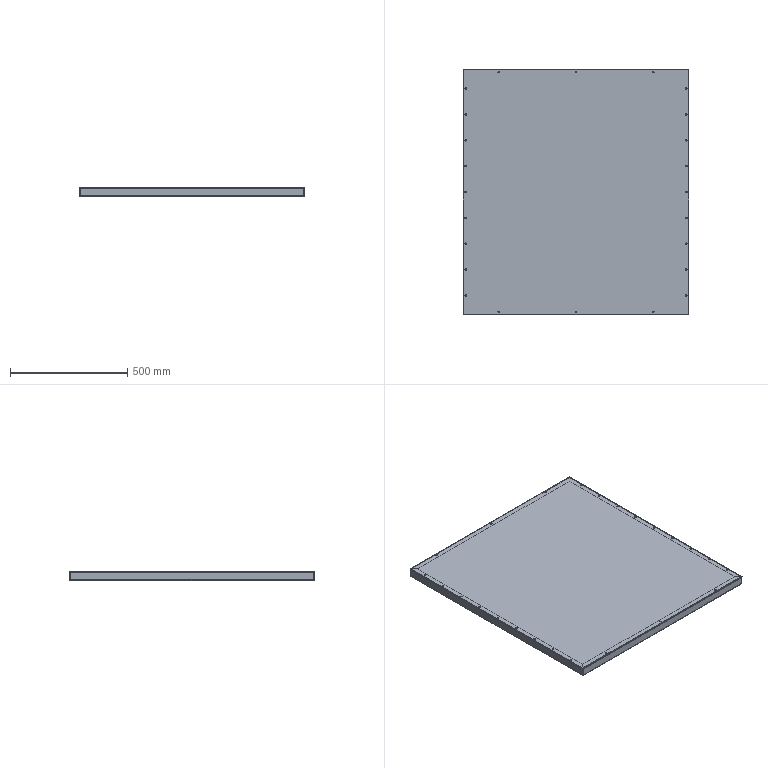Part | SolidWorks | 2 solids | 172 faces | box 962 x 1043 x 39 mm | volume 5034136 mm3 | cylinder 112 | plane 44 | spline 16 | commonest cylinder face diameters 5 x48 6.5 x48 1.473 x8 6.473 x8